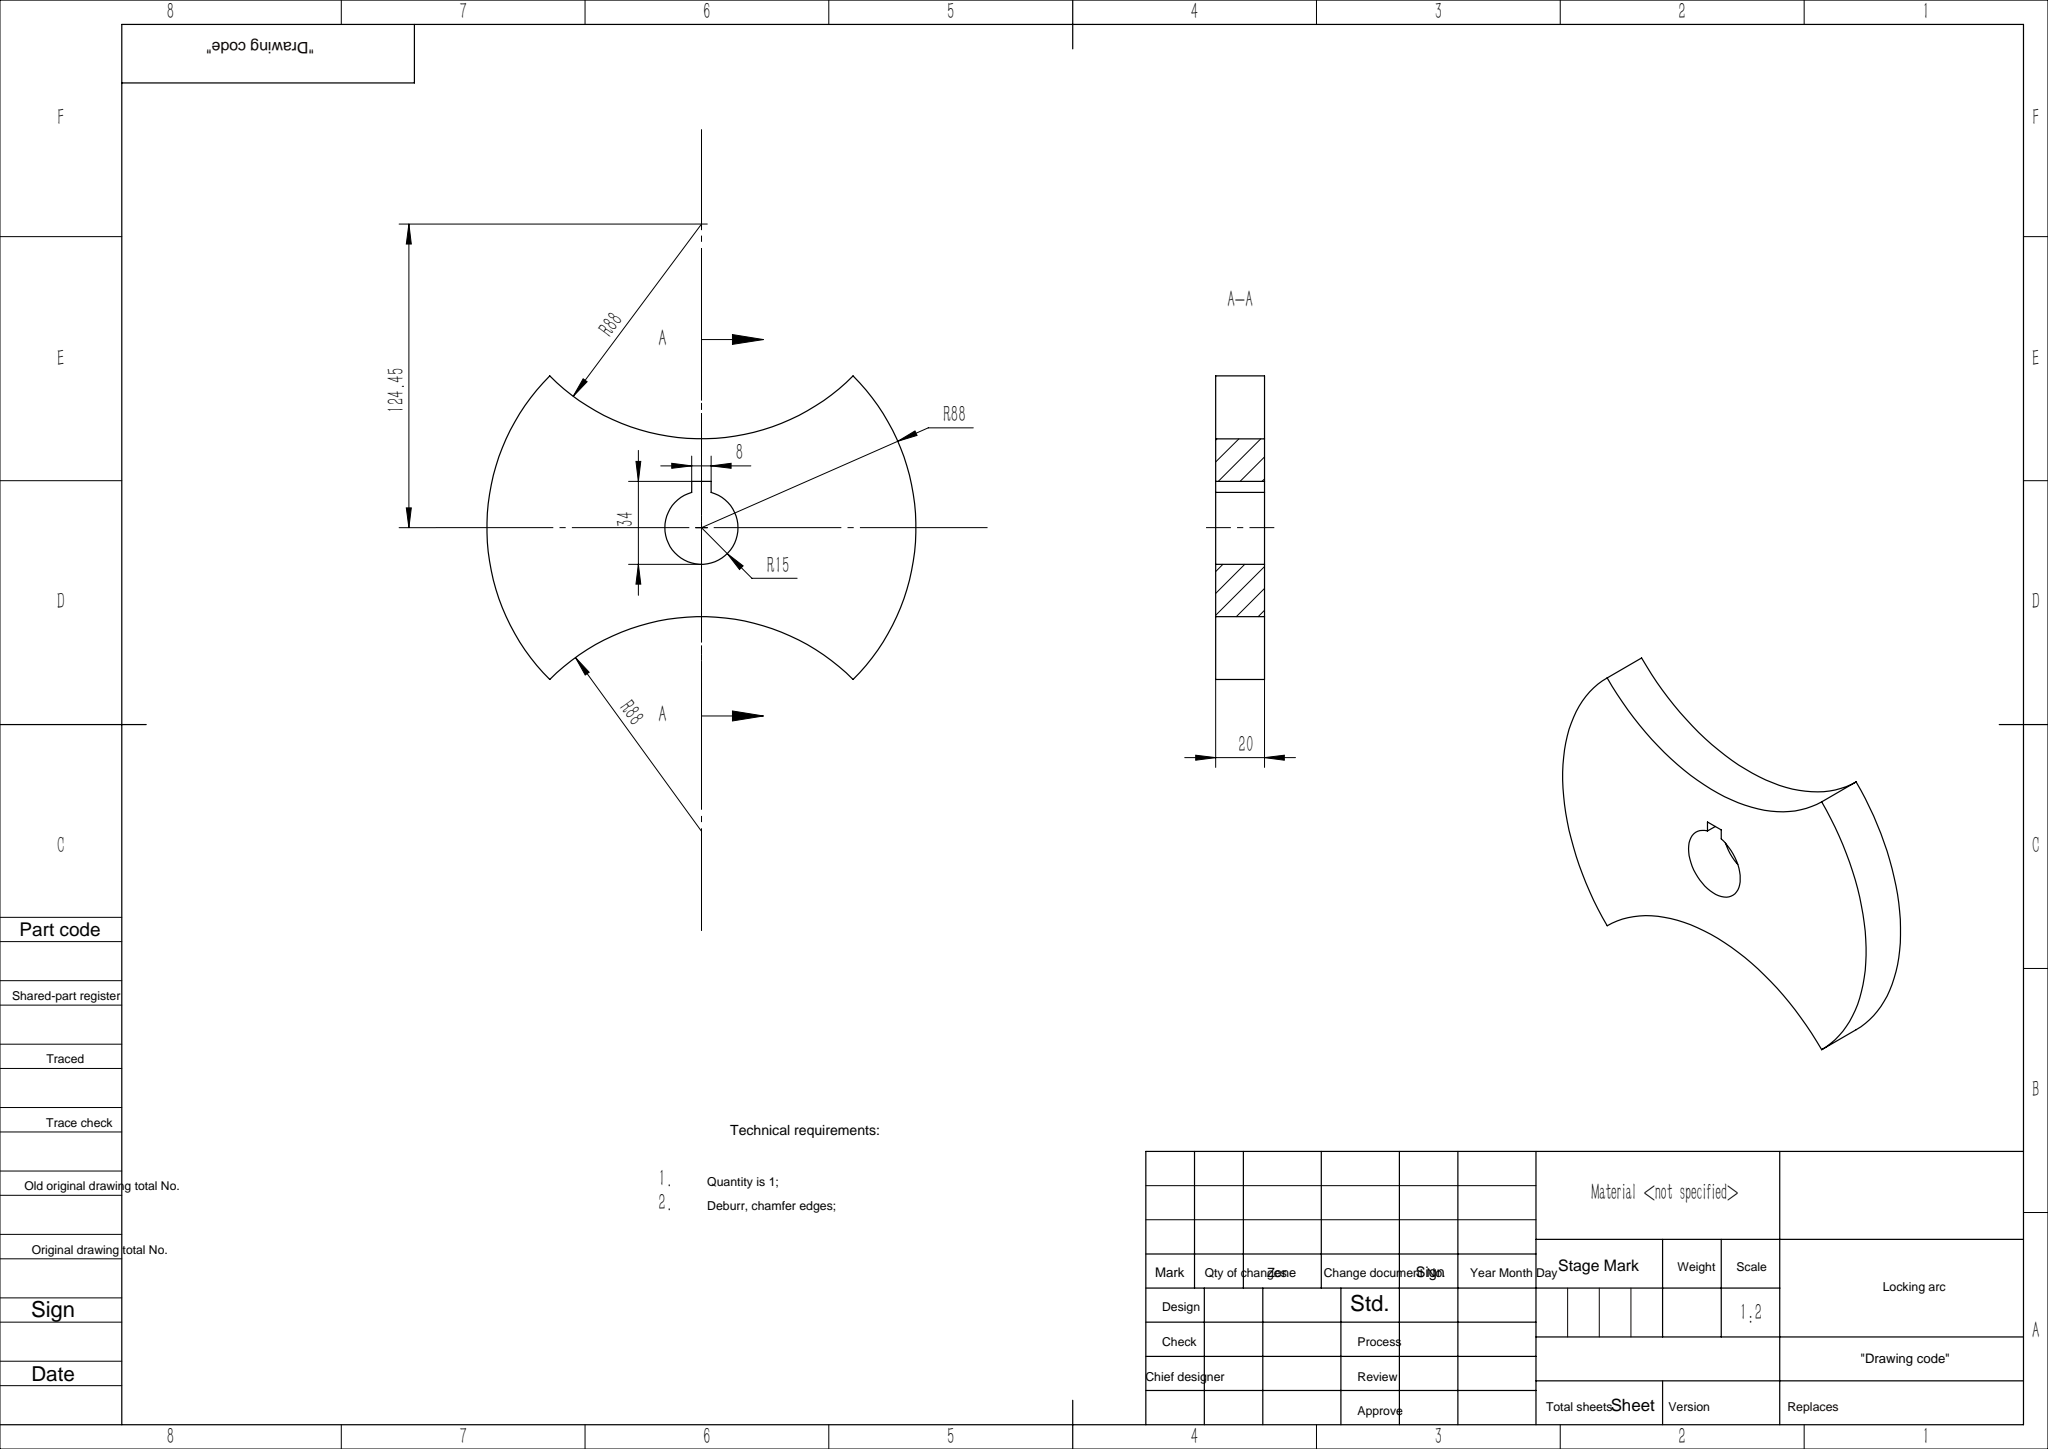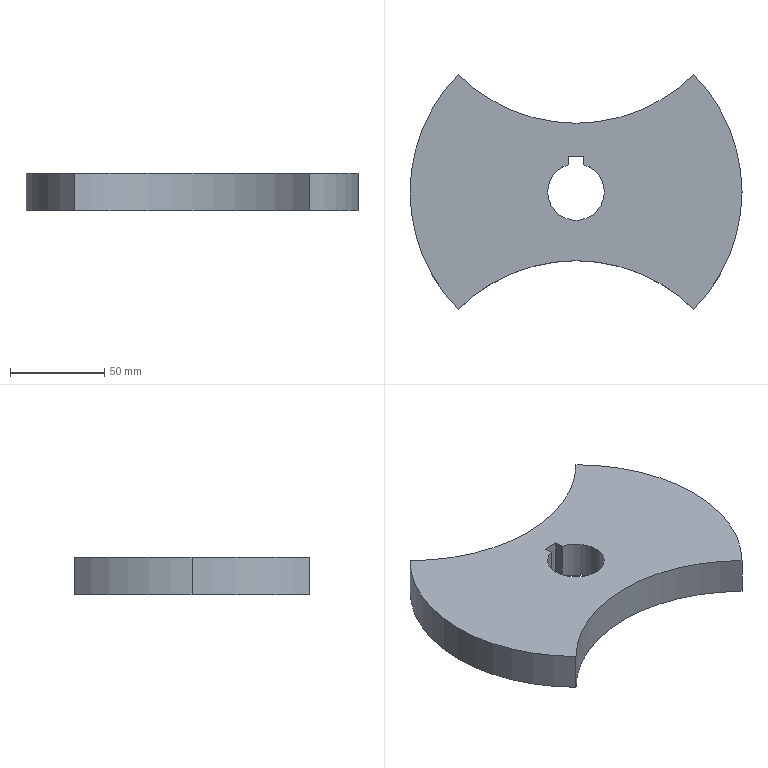Part | SolidWorks | features Extrusion 1, ICE 1 | 1 solid | 13 faces | box 176 x 124.451 x 20 mm | volume 294954 mm3 | cylinder 8 | plane 5 | commonest cylinder face diameters 176 x5 30 x3
STEP:
#1=CARTESIAN_POINT('',(-15.,0.,0.));
#2=VERTEX_POINT('',#1);
#3=CARTESIAN_POINT('',(15.,0.,0.));
#4=VERTEX_POINT('',#3);
#5=CARTESIAN_POINT('',(0.,0.,0.));
#6=DIRECTION('',(0.,0.,1.));
#7=DIRECTION('',(1.,0.,0.));
#8=AXIS2_PLACEMENT_3D('',#5,#6,#7);
#9=CIRCLE('',#8,15.);
#10=EDGE_CURVE('',#2,#4,#9,.T.);
#11=ORIENTED_EDGE('',*,*,#10,.F.);
#12=CARTESIAN_POINT('',(-15.,0.,20.));
#13=VERTEX_POINT('',#12);
#14=CARTESIAN_POINT('',(-15.,0.,0.));
#15=DIRECTION('',(0.,0.,1.));
#16=VECTOR('',#15,1000.);
#17=LINE('',#14,#16);
#18=EDGE_CURVE('',#2,#13,#17,.T.);
#19=ORIENTED_EDGE('',*,*,#18,.T.);
#20=CARTESIAN_POINT('',(15.,0.,20.));
#21=VERTEX_POINT('',#20);
#22=CARTESIAN_POINT('',(0.,0.,20.));
#23=DIRECTION('',(0.,0.,1.));
#24=DIRECTION('',(1.,0.,0.));
#25=AXIS2_PLACEMENT_3D('',#22,#23,#24);
#26=CIRCLE('',#25,15.);
#27=EDGE_CURVE('',#13,#21,#26,.T.);
#28=ORIENTED_EDGE('',*,*,#27,.T.);
#29=CARTESIAN_POINT('',(15.,0.,0.));
#30=DIRECTION('',(0.,0.,1.));
#31=VECTOR('',#30,1000.);
#32=LINE('',#29,#31);
#33=EDGE_CURVE('',#4,#21,#32,.T.);
#34=ORIENTED_EDGE('',*,*,#33,.F.);
#35=EDGE_LOOP('',(#11,#19,#28,#34));
#36=FACE_OUTER_BOUND('',#35,.T.);
#37=CARTESIAN_POINT('',(0.,0.,0.));
#38=DIRECTION('',(0.,0.,1.));
#39=DIRECTION('',(1.,0.,0.));
#40=AXIS2_PLACEMENT_3D('',#37,#38,#39);
#41=CYLINDRICAL_SURFACE('',#40,15.);
#42=ADVANCED_FACE('',(#36),#41,.F.);
#43=CARTESIAN_POINT('',(4.,14.457,0.));
#44=VERTEX_POINT('',#43);
#45=CARTESIAN_POINT('',(0.,0.,0.));
#46=DIRECTION('',(0.,0.,1.));
#47=DIRECTION('',(1.,0.,0.));
#48=AXIS2_PLACEMENT_3D('',#45,#46,#47);
#49=CIRCLE('',#48,15.);
#50=EDGE_CURVE('',#4,#44,#49,.T.);
#51=ORIENTED_EDGE('',*,*,#50,.F.);
#52=ORIENTED_EDGE('',*,*,#33,.T.);
#53=CARTESIAN_POINT('',(4.,14.457,20.));
#54=VERTEX_POINT('',#53);
#55=CARTESIAN_POINT('',(0.,0.,20.));
#56=DIRECTION('',(0.,0.,1.));
#57=DIRECTION('',(1.,0.,0.));
#58=AXIS2_PLACEMENT_3D('',#55,#56,#57);
#59=CIRCLE('',#58,15.);
#60=EDGE_CURVE('',#21,#54,#59,.T.);
#61=ORIENTED_EDGE('',*,*,#60,.T.);
#62=CARTESIAN_POINT('',(4.,14.457,0.));
#63=DIRECTION('',(0.,0.,1.));
#64=VECTOR('',#63,1000.);
#65=LINE('',#62,#64);
#66=EDGE_CURVE('',#44,#54,#65,.T.);
#67=ORIENTED_EDGE('',*,*,#66,.F.);
#68=EDGE_LOOP('',(#51,#52,#61,#67));
#69=FACE_OUTER_BOUND('',#68,.T.);
#70=CARTESIAN_POINT('',(0.,0.,0.));
#71=DIRECTION('',(0.,0.,1.));
#72=DIRECTION('',(1.,0.,0.));
#73=AXIS2_PLACEMENT_3D('',#70,#71,#72);
#74=CYLINDRICAL_SURFACE('',#73,15.);
#75=ADVANCED_FACE('',(#69),#74,.F.);
#76=CARTESIAN_POINT('',(-88.,0.,20.));
#77=VERTEX_POINT('',#76);
#78=CARTESIAN_POINT('',(-62.225,-62.225,20.));
#79=VERTEX_POINT('',#78);
#80=CARTESIAN_POINT('',(0.,0.,20.));
#81=DIRECTION('',(0.,0.,1.));
#82=DIRECTION('',(1.,0.,0.));
#83=AXIS2_PLACEMENT_3D('',#80,#81,#82);
#84=CIRCLE('',#83,88.);
#85=EDGE_CURVE('',#77,#79,#84,.T.);
#86=ORIENTED_EDGE('',*,*,#85,.F.);
#87=CARTESIAN_POINT('',(-88.,0.,0.));
#88=VERTEX_POINT('',#87);
#89=CARTESIAN_POINT('',(-88.,0.,20.));
#90=DIRECTION('',(0.,0.,-1.));
#91=VECTOR('',#90,1000.);
#92=LINE('',#89,#91);
#93=EDGE_CURVE('',#77,#88,#92,.T.);
#94=ORIENTED_EDGE('',*,*,#93,.T.);
#95=CARTESIAN_POINT('',(-62.225,-62.225,0.));
#96=VERTEX_POINT('',#95);
#97=CARTESIAN_POINT('',(0.,0.,0.));
#98=DIRECTION('',(0.,0.,1.));
#99=DIRECTION('',(1.,0.,0.));
#100=AXIS2_PLACEMENT_3D('',#97,#98,#99);
#101=CIRCLE('',#100,88.);
#102=EDGE_CURVE('',#88,#96,#101,.T.);
#103=ORIENTED_EDGE('',*,*,#102,.T.);
#104=CARTESIAN_POINT('',(-62.225,-62.225,20.));
#105=DIRECTION('',(0.,0.,-1.));
#106=VECTOR('',#105,1000.);
#107=LINE('',#104,#106);
#108=EDGE_CURVE('',#79,#96,#107,.T.);
#109=ORIENTED_EDGE('',*,*,#108,.F.);
#110=EDGE_LOOP('',(#86,#94,#103,#109));
#111=FACE_OUTER_BOUND('',#110,.T.);
#112=CARTESIAN_POINT('',(0.,0.,20.));
#113=DIRECTION('',(0.,0.,-1.));
#114=DIRECTION('',(-1.,0.,0.));
#115=AXIS2_PLACEMENT_3D('',#112,#113,#114);
#116=CYLINDRICAL_SURFACE('',#115,88.);
#117=ADVANCED_FACE('',(#111),#116,.T.);
#118=CARTESIAN_POINT('',(62.225,-62.225,0.));
#119=VERTEX_POINT('',#118);
#120=CARTESIAN_POINT('',(0.,-124.451,0.));
#121=DIRECTION('',(0.,0.,-1.));
#122=DIRECTION('',(-1.,0.,0.));
#123=AXIS2_PLACEMENT_3D('',#120,#121,#122);
#124=CIRCLE('',#123,88.);
#125=EDGE_CURVE('',#96,#119,#124,.T.);
#126=ORIENTED_EDGE('',*,*,#125,.T.);
#127=CARTESIAN_POINT('',(62.225,-62.225,20.));
#128=VERTEX_POINT('',#127);
#129=CARTESIAN_POINT('',(62.225,-62.225,20.));
#130=DIRECTION('',(0.,0.,-1.));
#131=VECTOR('',#130,1000.);
#132=LINE('',#129,#131);
#133=EDGE_CURVE('',#128,#119,#132,.T.);
#134=ORIENTED_EDGE('',*,*,#133,.F.);
#135=CARTESIAN_POINT('',(0.,-124.451,20.));
#136=DIRECTION('',(0.,0.,-1.));
#137=DIRECTION('',(-1.,0.,0.));
#138=AXIS2_PLACEMENT_3D('',#135,#136,#137);
#139=CIRCLE('',#138,88.);
#140=EDGE_CURVE('',#79,#128,#139,.T.);
#141=ORIENTED_EDGE('',*,*,#140,.F.);
#142=ORIENTED_EDGE('',*,*,#108,.T.);
#143=EDGE_LOOP('',(#126,#134,#141,#142));
#144=FACE_OUTER_BOUND('',#143,.T.);
#145=CARTESIAN_POINT('',(0.,-124.451,20.));
#146=DIRECTION('',(0.,0.,-1.));
#147=DIRECTION('',(-1.,0.,0.));
#148=AXIS2_PLACEMENT_3D('',#145,#146,#147);
#149=CYLINDRICAL_SURFACE('',#148,88.);
#150=ADVANCED_FACE('',(#144),#149,.F.);
#151=CARTESIAN_POINT('',(62.225,62.225,0.));
#152=VERTEX_POINT('',#151);
#153=CARTESIAN_POINT('',(0.,0.,0.));
#154=DIRECTION('',(0.,0.,1.));
#155=DIRECTION('',(1.,0.,0.));
#156=AXIS2_PLACEMENT_3D('',#153,#154,#155);
#157=CIRCLE('',#156,88.);
#158=EDGE_CURVE('',#119,#152,#157,.T.);
#159=ORIENTED_EDGE('',*,*,#158,.T.);
#160=CARTESIAN_POINT('',(62.225,62.225,20.));
#161=VERTEX_POINT('',#160);
#162=CARTESIAN_POINT('',(62.225,62.225,20.));
#163=DIRECTION('',(0.,0.,-1.));
#164=VECTOR('',#163,1000.);
#165=LINE('',#162,#164);
#166=EDGE_CURVE('',#161,#152,#165,.T.);
#167=ORIENTED_EDGE('',*,*,#166,.F.);
#168=CARTESIAN_POINT('',(0.,0.,20.));
#169=DIRECTION('',(0.,0.,1.));
#170=DIRECTION('',(1.,0.,0.));
#171=AXIS2_PLACEMENT_3D('',#168,#169,#170);
#172=CIRCLE('',#171,88.);
#173=EDGE_CURVE('',#128,#161,#172,.T.);
#174=ORIENTED_EDGE('',*,*,#173,.F.);
#175=ORIENTED_EDGE('',*,*,#133,.T.);
#176=EDGE_LOOP('',(#159,#167,#174,#175));
#177=FACE_OUTER_BOUND('',#176,.T.);
#178=CARTESIAN_POINT('',(0.,0.,20.));
#179=DIRECTION('',(0.,0.,-1.));
#180=DIRECTION('',(-1.,0.,0.));
#181=AXIS2_PLACEMENT_3D('',#178,#179,#180);
#182=CYLINDRICAL_SURFACE('',#181,88.);
#183=ADVANCED_FACE('',(#177),#182,.T.);
#184=CARTESIAN_POINT('',(-62.225,62.225,0.));
#185=VERTEX_POINT('',#184);
#186=CARTESIAN_POINT('',(0.,124.451,0.));
#187=DIRECTION('',(0.,0.,-1.));
#188=DIRECTION('',(1.,0.,0.));
#189=AXIS2_PLACEMENT_3D('',#186,#187,#188);
#190=CIRCLE('',#189,88.);
#191=EDGE_CURVE('',#152,#185,#190,.T.);
#192=ORIENTED_EDGE('',*,*,#191,.T.);
#193=CARTESIAN_POINT('',(-62.225,62.225,20.));
#194=VERTEX_POINT('',#193);
#195=CARTESIAN_POINT('',(-62.225,62.225,20.));
#196=DIRECTION('',(0.,0.,-1.));
#197=VECTOR('',#196,1000.);
#198=LINE('',#195,#197);
#199=EDGE_CURVE('',#194,#185,#198,.T.);
#200=ORIENTED_EDGE('',*,*,#199,.F.);
#201=CARTESIAN_POINT('',(0.,124.451,20.));
#202=DIRECTION('',(0.,0.,-1.));
#203=DIRECTION('',(1.,0.,0.));
#204=AXIS2_PLACEMENT_3D('',#201,#202,#203);
#205=CIRCLE('',#204,88.);
#206=EDGE_CURVE('',#161,#194,#205,.T.);
#207=ORIENTED_EDGE('',*,*,#206,.F.);
#208=ORIENTED_EDGE('',*,*,#166,.T.);
#209=EDGE_LOOP('',(#192,#200,#207,#208));
#210=FACE_OUTER_BOUND('',#209,.T.);
#211=CARTESIAN_POINT('',(0.,124.451,20.));
#212=DIRECTION('',(0.,0.,-1.));
#213=DIRECTION('',(-1.,0.,0.));
#214=AXIS2_PLACEMENT_3D('',#211,#212,#213);
#215=CYLINDRICAL_SURFACE('',#214,88.);
#216=ADVANCED_FACE('',(#210),#215,.F.);
#217=ORIENTED_EDGE('',*,*,#93,.F.);
#218=CARTESIAN_POINT('',(0.,0.,20.));
#219=DIRECTION('',(0.,0.,1.));
#220=DIRECTION('',(1.,0.,0.));
#221=AXIS2_PLACEMENT_3D('',#218,#219,#220);
#222=CIRCLE('',#221,88.);
#223=EDGE_CURVE('',#194,#77,#222,.T.);
#224=ORIENTED_EDGE('',*,*,#223,.F.);
#225=ORIENTED_EDGE('',*,*,#199,.T.);
#226=CARTESIAN_POINT('',(0.,0.,0.));
#227=DIRECTION('',(0.,0.,1.));
#228=DIRECTION('',(1.,0.,0.));
#229=AXIS2_PLACEMENT_3D('',#226,#227,#228);
#230=CIRCLE('',#229,88.);
#231=EDGE_CURVE('',#185,#88,#230,.T.);
#232=ORIENTED_EDGE('',*,*,#231,.T.);
#233=EDGE_LOOP('',(#217,#224,#225,#232));
#234=FACE_OUTER_BOUND('',#233,.T.);
#235=CARTESIAN_POINT('',(0.,0.,20.));
#236=DIRECTION('',(0.,0.,-1.));
#237=DIRECTION('',(-1.,0.,0.));
#238=AXIS2_PLACEMENT_3D('',#235,#236,#237);
#239=CYLINDRICAL_SURFACE('',#238,88.);
#240=ADVANCED_FACE('',(#234),#239,.T.);
#241=CARTESIAN_POINT('',(4.,19.,20.));
#242=VERTEX_POINT('',#241);
#243=CARTESIAN_POINT('',(4.,19.,20.));
#244=DIRECTION('',(0.,1.,0.));
#245=VECTOR('',#244,1000.);
#246=LINE('',#243,#245);
#247=EDGE_CURVE('',#54,#242,#246,.T.);
#248=ORIENTED_EDGE('',*,*,#247,.F.);
#249=ORIENTED_EDGE('',*,*,#60,.F.);
#250=ORIENTED_EDGE('',*,*,#27,.F.);
#251=CARTESIAN_POINT('',(-4.,14.457,20.));
#252=VERTEX_POINT('',#251);
#253=CARTESIAN_POINT('',(0.,0.,20.));
#254=DIRECTION('',(0.,0.,1.));
#255=DIRECTION('',(1.,0.,0.));
#256=AXIS2_PLACEMENT_3D('',#253,#254,#255);
#257=CIRCLE('',#256,15.);
#258=EDGE_CURVE('',#252,#13,#257,.T.);
#259=ORIENTED_EDGE('',*,*,#258,.F.);
#260=CARTESIAN_POINT('',(-4.,19.,20.));
#261=VERTEX_POINT('',#260);
#262=CARTESIAN_POINT('',(-4.,19.,20.));
#263=DIRECTION('',(0.,-1.,0.));
#264=VECTOR('',#263,1000.);
#265=LINE('',#262,#264);
#266=EDGE_CURVE('',#261,#252,#265,.T.);
#267=ORIENTED_EDGE('',*,*,#266,.F.);
#268=CARTESIAN_POINT('',(-4.,19.,20.));
#269=DIRECTION('',(-1.,0.,0.));
#270=VECTOR('',#269,1000.);
#271=LINE('',#268,#270);
#272=EDGE_CURVE('',#242,#261,#271,.T.);
#273=ORIENTED_EDGE('',*,*,#272,.F.);
#274=EDGE_LOOP('',(#248,#249,#250,#259,#267,#273));
#275=FACE_BOUND('',#274,.T.);
#276=ORIENTED_EDGE('',*,*,#140,.T.);
#277=ORIENTED_EDGE('',*,*,#173,.T.);
#278=ORIENTED_EDGE('',*,*,#206,.T.);
#279=ORIENTED_EDGE('',*,*,#223,.T.);
#280=ORIENTED_EDGE('',*,*,#85,.T.);
#281=EDGE_LOOP('',(#276,#277,#278,#279,#280));
#282=FACE_OUTER_BOUND('',#281,.T.);
#283=CARTESIAN_POINT('',(0.,-62.225,20.));
#284=DIRECTION('',(0.,0.,-1.));
#285=DIRECTION('',(-1.,0.,0.));
#286=AXIS2_PLACEMENT_3D('',#283,#284,#285);
#287=PLANE('',#286);
#288=ADVANCED_FACE('',(#275,#282),#287,.F.);
#289=CARTESIAN_POINT('',(-4.,14.457,0.));
#290=VERTEX_POINT('',#289);
#291=CARTESIAN_POINT('',(0.,0.,0.));
#292=DIRECTION('',(0.,0.,1.));
#293=DIRECTION('',(1.,0.,0.));
#294=AXIS2_PLACEMENT_3D('',#291,#292,#293);
#295=CIRCLE('',#294,15.);
#296=EDGE_CURVE('',#290,#2,#295,.T.);
#297=ORIENTED_EDGE('',*,*,#296,.T.);
#298=ORIENTED_EDGE('',*,*,#10,.T.);
#299=ORIENTED_EDGE('',*,*,#50,.T.);
#300=CARTESIAN_POINT('',(4.,19.,0.));
#301=VERTEX_POINT('',#300);
#302=CARTESIAN_POINT('',(4.,19.,0.));
#303=DIRECTION('',(0.,1.,0.));
#304=VECTOR('',#303,1000.);
#305=LINE('',#302,#304);
#306=EDGE_CURVE('',#44,#301,#305,.T.);
#307=ORIENTED_EDGE('',*,*,#306,.T.);
#308=CARTESIAN_POINT('',(-4.,19.,0.));
#309=VERTEX_POINT('',#308);
#310=CARTESIAN_POINT('',(-4.,19.,0.));
#311=DIRECTION('',(-1.,0.,0.));
#312=VECTOR('',#311,1000.);
#313=LINE('',#310,#312);
#314=EDGE_CURVE('',#301,#309,#313,.T.);
#315=ORIENTED_EDGE('',*,*,#314,.T.);
#316=CARTESIAN_POINT('',(-4.,19.,0.));
#317=DIRECTION('',(0.,-1.,0.));
#318=VECTOR('',#317,1000.);
#319=LINE('',#316,#318);
#320=EDGE_CURVE('',#309,#290,#319,.T.);
#321=ORIENTED_EDGE('',*,*,#320,.T.);
#322=EDGE_LOOP('',(#297,#298,#299,#307,#315,#321));
#323=FACE_BOUND('',#322,.T.);
#324=ORIENTED_EDGE('',*,*,#125,.F.);
#325=ORIENTED_EDGE('',*,*,#102,.F.);
#326=ORIENTED_EDGE('',*,*,#231,.F.);
#327=ORIENTED_EDGE('',*,*,#191,.F.);
#328=ORIENTED_EDGE('',*,*,#158,.F.);
#329=EDGE_LOOP('',(#324,#325,#326,#327,#328));
#330=FACE_OUTER_BOUND('',#329,.T.);
#331=CARTESIAN_POINT('',(0.,-62.225,0.));
#332=DIRECTION('',(0.,0.,-1.));
#333=DIRECTION('',(-1.,0.,0.));
#334=AXIS2_PLACEMENT_3D('',#331,#332,#333);
#335=PLANE('',#334);
#336=ADVANCED_FACE('',(#323,#330),#335,.T.);
#337=ORIENTED_EDGE('',*,*,#18,.F.);
#338=ORIENTED_EDGE('',*,*,#296,.F.);
#339=CARTESIAN_POINT('',(-4.,14.457,0.));
#340=DIRECTION('',(0.,0.,1.));
#341=VECTOR('',#340,1000.);
#342=LINE('',#339,#341);
#343=EDGE_CURVE('',#290,#252,#342,.T.);
#344=ORIENTED_EDGE('',*,*,#343,.T.);
#345=ORIENTED_EDGE('',*,*,#258,.T.);
#346=EDGE_LOOP('',(#337,#338,#344,#345));
#347=FACE_OUTER_BOUND('',#346,.T.);
#348=CARTESIAN_POINT('',(0.,0.,0.));
#349=DIRECTION('',(0.,0.,1.));
#350=DIRECTION('',(1.,0.,0.));
#351=AXIS2_PLACEMENT_3D('',#348,#349,#350);
#352=CYLINDRICAL_SURFACE('',#351,15.);
#353=ADVANCED_FACE('',(#347),#352,.F.);
#354=ORIENTED_EDGE('',*,*,#266,.T.);
#355=ORIENTED_EDGE('',*,*,#343,.F.);
#356=ORIENTED_EDGE('',*,*,#320,.F.);
#357=CARTESIAN_POINT('',(-4.,19.,0.));
#358=DIRECTION('',(0.,0.,1.));
#359=VECTOR('',#358,1000.);
#360=LINE('',#357,#359);
#361=EDGE_CURVE('',#309,#261,#360,.T.);
#362=ORIENTED_EDGE('',*,*,#361,.T.);
#363=EDGE_LOOP('',(#354,#355,#356,#362));
#364=FACE_OUTER_BOUND('',#363,.T.);
#365=CARTESIAN_POINT('',(-4.,19.,0.));
#366=DIRECTION('',(-1.,0.,0.));
#367=DIRECTION('',(0.,0.,1.));
#368=AXIS2_PLACEMENT_3D('',#365,#366,#367);
#369=PLANE('',#368);
#370=ADVANCED_FACE('',(#364),#369,.F.);
#371=ORIENTED_EDGE('',*,*,#272,.T.);
#372=ORIENTED_EDGE('',*,*,#361,.F.);
#373=ORIENTED_EDGE('',*,*,#314,.F.);
#374=CARTESIAN_POINT('',(4.,19.,0.));
#375=DIRECTION('',(0.,0.,1.));
#376=VECTOR('',#375,1000.);
#377=LINE('',#374,#376);
#378=EDGE_CURVE('',#301,#242,#377,.T.);
#379=ORIENTED_EDGE('',*,*,#378,.T.);
#380=EDGE_LOOP('',(#371,#372,#373,#379));
#381=FACE_OUTER_BOUND('',#380,.T.);
#382=CARTESIAN_POINT('',(-4.,19.,0.));
#383=DIRECTION('',(0.,1.,0.));
#384=DIRECTION('',(0.,0.,1.));
#385=AXIS2_PLACEMENT_3D('',#382,#383,#384);
#386=PLANE('',#385);
#387=ADVANCED_FACE('',(#381),#386,.F.);
#388=ORIENTED_EDGE('',*,*,#247,.T.);
#389=ORIENTED_EDGE('',*,*,#378,.F.);
#390=ORIENTED_EDGE('',*,*,#306,.F.);
#391=ORIENTED_EDGE('',*,*,#66,.T.);
#392=EDGE_LOOP('',(#388,#389,#390,#391));
#393=FACE_OUTER_BOUND('',#392,.T.);
#394=CARTESIAN_POINT('',(4.,19.,0.));
#395=DIRECTION('',(1.,0.,0.));
#396=DIRECTION('',(0.,0.,-1.));
#397=AXIS2_PLACEMENT_3D('',#394,#395,#396);
#398=PLANE('',#397);
#399=ADVANCED_FACE('',(#393),#398,.F.);
#400=CLOSED_SHELL('',(#42,#75,#117,#150,#183,#216,#240,#288,#336,#353,#370,#387,#399));
#401=MANIFOLD_SOLID_BREP('',#400);
#402=CARTESIAN_POINT('',(0.,0.,0.));
#403=DIRECTION('',(0.,0.,1.));
#404=DIRECTION('',(1.,0.,0.));
#405=AXIS2_PLACEMENT_3D('',#402,#403,#404);
#406=(LENGTH_UNIT()NAMED_UNIT(*)SI_UNIT(.MILLI.,.METRE.));
#407=UNCERTAINTY_MEASURE_WITH_UNIT(LENGTH_MEASURE(0.00001),#406,'','');
#408=(NAMED_UNIT(*)PLANE_ANGLE_UNIT()SI_UNIT($,.RADIAN.));
#409=(NAMED_UNIT(*)SI_UNIT($,.STERADIAN.)SOLID_ANGLE_UNIT());
#410=(GEOMETRIC_REPRESENTATION_CONTEXT(3)GLOBAL_UNCERTAINTY_ASSIGNED_CONTEXT((#407))GLOBAL_UNIT_ASSIGNED_CONTEXT((#406,#408,#409))REPRESENTATION_CONTEXT('',''));
#411=ADVANCED_BREP_SHAPE_REPRESENTATION('',(#401,#405),#410);